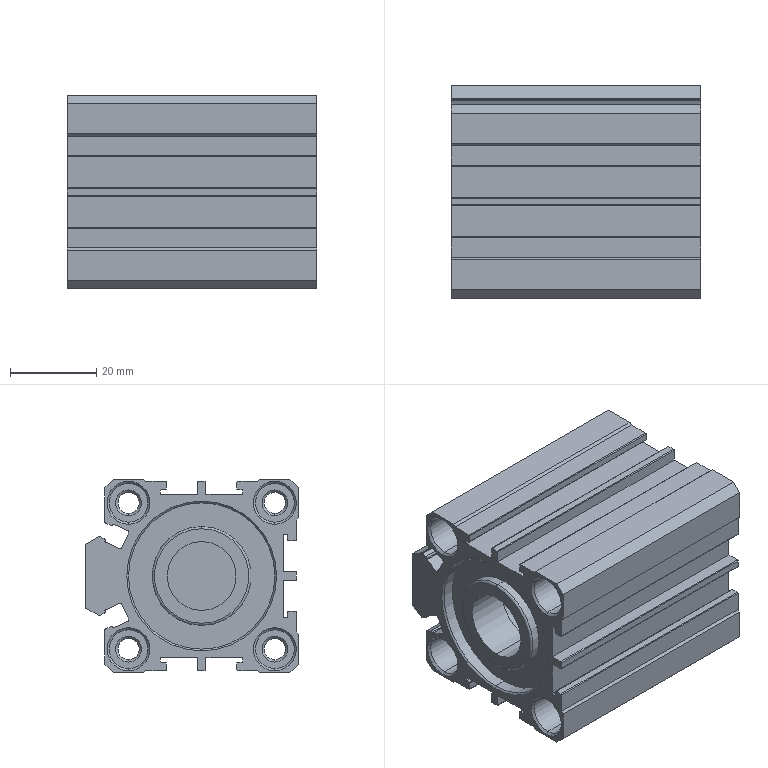Part | SolidWorks | features BaseBody 1 | 1 solid | 227 faces | box 58 x 49.5 x 45 mm | volume 61209 mm3 | cylinder 92 | plane 89 | cone 44 | torus 2 | commonest cylinder face diameters 0.4 x35 9 x16 0.8 x10 4.917 x8 8.566 x4 23 x4